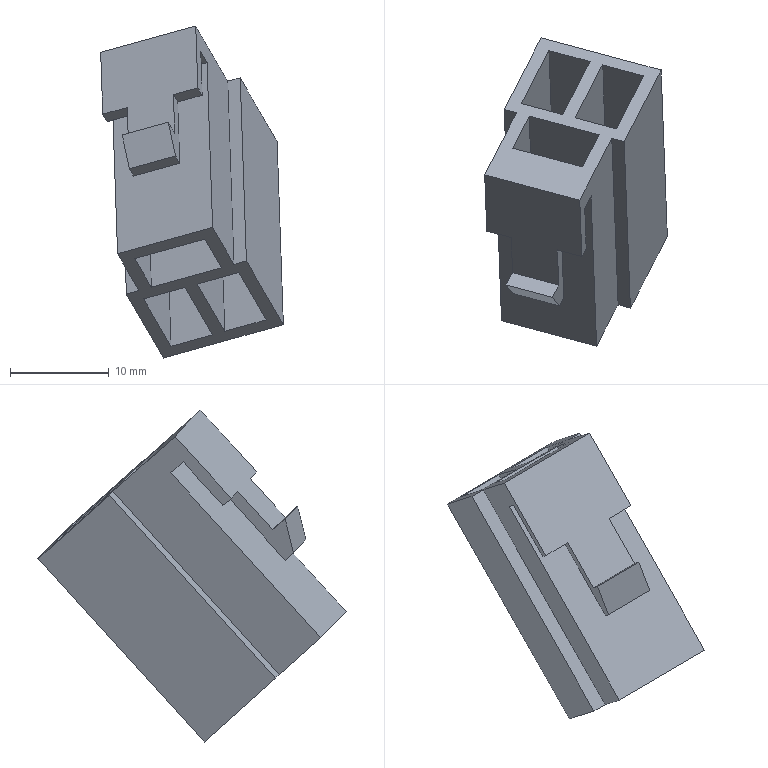Part | SolidWorks | features BaseBody 1 | 1 solid | 32 faces | box 18.462 x 31.146 x 33.559 mm | volume 2533 mm3 | plane 32
STEP:
#1=CARTESIAN_POINT('',(-173.307,-69.475,5.1));
#2=VERTEX_POINT('',#1);
#3=CARTESIAN_POINT('',(-173.175,-73.005,1.213));
#4=VERTEX_POINT('',#3);
#5=CARTESIAN_POINT('',(-173.175,-73.005,1.213));
#6=DIRECTION('',(0.02515,-0.6722,-0.7399));
#7=VECTOR('',#6,1000.);
#8=LINE('',#5,#7);
#9=EDGE_CURVE('',#2,#4,#8,.T.);
#10=ORIENTED_EDGE('',*,*,#9,.T.);
#11=CARTESIAN_POINT('',(-173.822,-74.26,2.331));
#12=VERTEX_POINT('',#11);
#13=CARTESIAN_POINT('',(-173.822,-74.26,2.331));
#14=DIRECTION('',(-0.359,-0.6969,0.6209));
#15=VECTOR('',#14,1000.);
#16=LINE('',#13,#15);
#17=EDGE_CURVE('',#4,#12,#16,.T.);
#18=ORIENTED_EDGE('',*,*,#17,.T.);
#19=CARTESIAN_POINT('',(-173.097,-75.101,-1.094));
#20=VERTEX_POINT('',#19);
#21=CARTESIAN_POINT('',(-173.097,-75.101,-1.094));
#22=DIRECTION('',(0.2013,-0.2337,-0.9513));
#23=VECTOR('',#22,1000.);
#24=LINE('',#21,#23);
#25=EDGE_CURVE('',#12,#20,#24,.T.);
#26=ORIENTED_EDGE('',*,*,#25,.T.);
#27=CARTESIAN_POINT('',(-172.666,-74.265,-1.839));
#28=VERTEX_POINT('',#27);
#29=CARTESIAN_POINT('',(-172.666,-74.265,-1.839));
#30=DIRECTION('',(0.359,0.6969,-0.6209));
#31=VECTOR('',#30,1000.);
#32=LINE('',#29,#31);
#33=EDGE_CURVE('',#20,#28,#32,.T.);
#34=ORIENTED_EDGE('',*,*,#33,.T.);
#35=CARTESIAN_POINT('',(-172.877,-68.639,4.355));
#36=VERTEX_POINT('',#35);
#37=CARTESIAN_POINT('',(-173.027,-64.617,8.781));
#38=DIRECTION('',(-0.02515,0.6722,0.7399));
#39=VECTOR('',#38,1000.);
#40=LINE('',#37,#39);
#41=EDGE_CURVE('',#28,#36,#40,.T.);
#42=ORIENTED_EDGE('',*,*,#41,.T.);
#43=CARTESIAN_POINT('',(-174.384,-71.565,6.963));
#44=DIRECTION('',(0.359,0.6969,-0.6209));
#45=VECTOR('',#44,1000.);
#46=LINE('',#43,#45);
#47=EDGE_CURVE('',#2,#36,#46,.T.);
#48=ORIENTED_EDGE('',*,*,#47,.F.);
#49=EDGE_LOOP('',(#10,#18,#26,#34,#42,#48));
#50=FACE_OUTER_BOUND('',#49,.T.);
#51=CARTESIAN_POINT('',(-174.103,-79.094,-1.325));
#52=DIRECTION('',(-0.933,0.25,-0.2588));
#53=DIRECTION('',(-0.2673,0.,0.9636));
#54=AXIS2_PLACEMENT_3D('',#51,#52,#53);
#55=PLANE('',#54);
#56=ADVANCED_FACE('',(#50),#55,.F.);
#57=CARTESIAN_POINT('',(-170.835,-70.137,5.786));
#58=VERTEX_POINT('',#57);
#59=CARTESIAN_POINT('',(-170.835,-70.137,5.786));
#60=DIRECTION('',(-0.933,0.25,-0.2588));
#61=VECTOR('',#60,1000.);
#62=LINE('',#59,#61);
#63=EDGE_CURVE('',#58,#2,#62,.T.);
#64=ORIENTED_EDGE('',*,*,#63,.T.);
#65=ORIENTED_EDGE('',*,*,#47,.T.);
#66=CARTESIAN_POINT('',(-170.404,-69.301,5.041));
#67=VERTEX_POINT('',#66);
#68=CARTESIAN_POINT('',(-170.404,-69.301,5.041));
#69=DIRECTION('',(0.933,-0.25,0.2588));
#70=VECTOR('',#69,1000.);
#71=LINE('',#68,#70);
#72=EDGE_CURVE('',#36,#67,#71,.T.);
#73=ORIENTED_EDGE('',*,*,#72,.T.);
#74=CARTESIAN_POINT('',(-169.758,-68.047,3.923));
#75=DIRECTION('',(0.359,0.6969,-0.6209));
#76=VECTOR('',#75,1000.);
#77=LINE('',#74,#76);
#78=EDGE_CURVE('',#58,#67,#77,.T.);
#79=ORIENTED_EDGE('',*,*,#78,.F.);
#80=EDGE_LOOP('',(#64,#65,#73,#79));
#81=FACE_OUTER_BOUND('',#80,.T.);
#82=CARTESIAN_POINT('',(-174.384,-71.565,6.963));
#83=DIRECTION('',(-0.02515,0.6722,0.7399));
#84=DIRECTION('',(0.9993,0.03738,0.));
#85=AXIS2_PLACEMENT_3D('',#82,#83,#84);
#86=PLANE('',#85);
#87=ADVANCED_FACE('',(#81),#86,.F.);
#88=CARTESIAN_POINT('',(-180.445,-67.562,3.12));
#89=VERTEX_POINT('',#88);
#90=CARTESIAN_POINT('',(-180.014,-66.726,2.375));
#91=VERTEX_POINT('',#90);
#92=CARTESIAN_POINT('',(-177.214,-61.29,-2.468));
#93=DIRECTION('',(0.359,0.6969,-0.6209));
#94=VECTOR('',#93,1000.);
#95=LINE('',#92,#94);
#96=EDGE_CURVE('',#89,#91,#95,.T.);
#97=ORIENTED_EDGE('',*,*,#96,.T.);
#98=CARTESIAN_POINT('',(-177.542,-67.389,3.061));
#99=VERTEX_POINT('',#98);
#100=CARTESIAN_POINT('',(-170.404,-69.301,5.041));
#101=DIRECTION('',(-0.933,0.25,-0.2588));
#102=VECTOR('',#101,1000.);
#103=LINE('',#100,#102);
#104=EDGE_CURVE('',#99,#91,#103,.T.);
#105=ORIENTED_EDGE('',*,*,#104,.F.);
#106=CARTESIAN_POINT('',(-177.973,-68.225,3.806));
#107=VERTEX_POINT('',#106);
#108=CARTESIAN_POINT('',(-179.049,-70.315,5.668));
#109=DIRECTION('',(0.359,0.6969,-0.6209));
#110=VECTOR('',#109,1000.);
#111=LINE('',#108,#110);
#112=EDGE_CURVE('',#107,#99,#111,.T.);
#113=ORIENTED_EDGE('',*,*,#112,.F.);
#114=CARTESIAN_POINT('',(-170.835,-70.137,5.786));
#115=DIRECTION('',(0.933,-0.25,0.2588));
#116=VECTOR('',#115,1000.);
#117=LINE('',#114,#116);
#118=EDGE_CURVE('',#89,#107,#117,.T.);
#119=ORIENTED_EDGE('',*,*,#118,.F.);
#120=EDGE_LOOP('',(#97,#105,#113,#119));
#121=FACE_OUTER_BOUND('',#120,.T.);
#122=CARTESIAN_POINT('',(-179.049,-70.315,5.668));
#123=DIRECTION('',(0.02515,-0.6722,-0.7399));
#124=DIRECTION('',(0.,-0.7402,0.6724));
#125=AXIS2_PLACEMENT_3D('',#122,#123,#124);
#126=PLANE('',#125);
#127=ADVANCED_FACE('',(#121),#126,.T.);
#128=ORIENTED_EDGE('',*,*,#112,.T.);
#129=CARTESIAN_POINT('',(-177.331,-73.015,-3.133));
#130=VERTEX_POINT('',#129);
#131=CARTESIAN_POINT('',(-177.692,-63.367,7.487));
#132=DIRECTION('',(-0.02515,0.6722,0.7399));
#133=VECTOR('',#132,1000.);
#134=LINE('',#131,#133);
#135=EDGE_CURVE('',#130,#99,#134,.T.);
#136=ORIENTED_EDGE('',*,*,#135,.F.);
#137=CARTESIAN_POINT('',(-177.762,-73.851,-2.388));
#138=VERTEX_POINT('',#137);
#139=CARTESIAN_POINT('',(-177.331,-73.015,-3.133));
#140=DIRECTION('',(0.359,0.6969,-0.6209));
#141=VECTOR('',#140,1000.);
#142=LINE('',#139,#141);
#143=EDGE_CURVE('',#138,#130,#142,.T.);
#144=ORIENTED_EDGE('',*,*,#143,.F.);
#145=CARTESIAN_POINT('',(-178.487,-73.01,1.037));
#146=VERTEX_POINT('',#145);
#147=CARTESIAN_POINT('',(-177.762,-73.851,-2.388));
#148=DIRECTION('',(0.2013,-0.2337,-0.9513));
#149=VECTOR('',#148,1000.);
#150=LINE('',#147,#149);
#151=EDGE_CURVE('',#146,#138,#150,.T.);
#152=ORIENTED_EDGE('',*,*,#151,.F.);
#153=CARTESIAN_POINT('',(-177.84,-71.755,-0.08074));
#154=VERTEX_POINT('',#153);
#155=CARTESIAN_POINT('',(-178.487,-73.01,1.037));
#156=DIRECTION('',(-0.359,-0.6969,0.6209));
#157=VECTOR('',#156,1000.);
#158=LINE('',#155,#157);
#159=EDGE_CURVE('',#154,#146,#158,.T.);
#160=ORIENTED_EDGE('',*,*,#159,.F.);
#161=CARTESIAN_POINT('',(-177.84,-71.755,-0.08074));
#162=DIRECTION('',(0.02515,-0.6722,-0.7399));
#163=VECTOR('',#162,1000.);
#164=LINE('',#161,#163);
#165=EDGE_CURVE('',#107,#154,#164,.T.);
#166=ORIENTED_EDGE('',*,*,#165,.F.);
#167=EDGE_LOOP('',(#128,#136,#144,#152,#160,#166));
#168=FACE_OUTER_BOUND('',#167,.T.);
#169=CARTESIAN_POINT('',(-178.768,-77.844,-2.619));
#170=DIRECTION('',(-0.933,0.25,-0.2588));
#171=DIRECTION('',(-0.2673,0.,0.9636));
#172=AXIS2_PLACEMENT_3D('',#169,#170,#171);
#173=PLANE('',#172);
#174=ADVANCED_FACE('',(#168),#173,.T.);
#175=CARTESIAN_POINT('',(-179.519,-61.45,5.684));
#176=VERTEX_POINT('',#175);
#177=CARTESIAN_POINT('',(-180.165,-62.705,6.801));
#178=VERTEX_POINT('',#177);
#179=CARTESIAN_POINT('',(-179.519,-61.45,5.684));
#180=DIRECTION('',(-0.359,-0.6969,0.6209));
#181=VECTOR('',#180,1000.);
#182=LINE('',#179,#181);
#183=EDGE_CURVE('',#176,#178,#182,.T.);
#184=ORIENTED_EDGE('',*,*,#183,.F.);
#185=CARTESIAN_POINT('',(-169.909,-64.025,8.35));
#186=VERTEX_POINT('',#185);
#187=CARTESIAN_POINT('',(-169.909,-64.025,8.35));
#188=DIRECTION('',(-0.933,0.25,-0.2588));
#189=VECTOR('',#188,1000.);
#190=LINE('',#187,#189);
#191=EDGE_CURVE('',#186,#176,#190,.T.);
#192=ORIENTED_EDGE('',*,*,#191,.F.);
#193=CARTESIAN_POINT('',(-170.555,-65.28,9.467));
#194=VERTEX_POINT('',#193);
#195=CARTESIAN_POINT('',(-169.909,-64.025,8.35));
#196=DIRECTION('',(-0.359,-0.6969,0.6209));
#197=VECTOR('',#196,1000.);
#198=LINE('',#195,#197);
#199=EDGE_CURVE('',#186,#194,#198,.T.);
#200=ORIENTED_EDGE('',*,*,#199,.T.);
#201=CARTESIAN_POINT('',(-170.555,-65.28,9.467));
#202=DIRECTION('',(-0.933,0.25,-0.2588));
#203=VECTOR('',#202,1000.);
#204=LINE('',#201,#203);
#205=EDGE_CURVE('',#194,#178,#204,.T.);
#206=ORIENTED_EDGE('',*,*,#205,.T.);
#207=EDGE_LOOP('',(#184,#192,#200,#206));
#208=FACE_OUTER_BOUND('',#207,.T.);
#209=CARTESIAN_POINT('',(-169.909,-64.025,8.35));
#210=DIRECTION('',(0.02515,-0.6722,-0.7399));
#211=DIRECTION('',(0.,-0.7402,0.6724));
#212=AXIS2_PLACEMENT_3D('',#209,#210,#211);
#213=PLANE('',#212);
#214=ADVANCED_FACE('',(#208),#213,.T.);
#215=CARTESIAN_POINT('',(-170.117,-77.892,-9.509));
#216=VERTEX_POINT('',#215);
#217=CARTESIAN_POINT('',(-168.448,-74.651,-12.396));
#218=VERTEX_POINT('',#217);
#219=CARTESIAN_POINT('',(-170.117,-77.892,-9.509));
#220=DIRECTION('',(0.359,0.6969,-0.6209));
#221=VECTOR('',#220,1000.);
#222=LINE('',#219,#221);
#223=EDGE_CURVE('',#216,#218,#222,.T.);
#224=ORIENTED_EDGE('',*,*,#223,.T.);
#225=CARTESIAN_POINT('',(-175.539,-72.751,-14.363));
#226=VERTEX_POINT('',#225);
#227=CARTESIAN_POINT('',(-168.448,-74.651,-12.396));
#228=DIRECTION('',(-0.933,0.25,-0.2588));
#229=VECTOR('',#228,1000.);
#230=LINE('',#227,#229);
#231=EDGE_CURVE('',#218,#226,#230,.T.);
#232=ORIENTED_EDGE('',*,*,#231,.T.);
#233=CARTESIAN_POINT('',(-177.208,-75.992,-11.476));
#234=VERTEX_POINT('',#233);
#235=CARTESIAN_POINT('',(-175.539,-72.751,-14.363));
#236=DIRECTION('',(-0.359,-0.6969,0.6209));
#237=VECTOR('',#236,1000.);
#238=LINE('',#235,#237);
#239=EDGE_CURVE('',#226,#234,#238,.T.);
#240=ORIENTED_EDGE('',*,*,#239,.T.);
#241=CARTESIAN_POINT('',(-177.208,-75.992,-11.476));
#242=DIRECTION('',(0.933,-0.25,0.2588));
#243=VECTOR('',#242,1000.);
#244=LINE('',#241,#243);
#245=EDGE_CURVE('',#234,#216,#244,.T.);
#246=ORIENTED_EDGE('',*,*,#245,.T.);
#247=EDGE_LOOP('',(#224,#232,#240,#246));
#248=FACE_BOUND('',#247,.T.);
#249=CARTESIAN_POINT('',(-169.374,-67.226,-19.173));
#250=VERTEX_POINT('',#249);
#251=CARTESIAN_POINT('',(-173.55,-66.107,-20.331));
#252=VERTEX_POINT('',#251);
#253=CARTESIAN_POINT('',(-169.374,-67.226,-19.173));
#254=DIRECTION('',(-0.933,0.25,-0.2588));
#255=VECTOR('',#254,1000.);
#256=LINE('',#253,#255);
#257=EDGE_CURVE('',#250,#252,#256,.T.);
#258=ORIENTED_EDGE('',*,*,#257,.T.);
#259=CARTESIAN_POINT('',(-176.314,-71.473,-15.551));
#260=VERTEX_POINT('',#259);
#261=CARTESIAN_POINT('',(-173.55,-66.107,-20.331));
#262=DIRECTION('',(-0.359,-0.6969,0.6209));
#263=VECTOR('',#262,1000.);
#264=LINE('',#261,#263);
#265=EDGE_CURVE('',#252,#260,#264,.T.);
#266=ORIENTED_EDGE('',*,*,#265,.T.);
#267=CARTESIAN_POINT('',(-172.138,-72.592,-14.392));
#268=VERTEX_POINT('',#267);
#269=CARTESIAN_POINT('',(-176.314,-71.473,-15.551));
#270=DIRECTION('',(0.933,-0.25,0.2588));
#271=VECTOR('',#270,1000.);
#272=LINE('',#269,#271);
#273=EDGE_CURVE('',#260,#268,#272,.T.);
#274=ORIENTED_EDGE('',*,*,#273,.T.);
#275=CARTESIAN_POINT('',(-172.138,-72.592,-14.392));
#276=DIRECTION('',(0.359,0.6969,-0.6209));
#277=VECTOR('',#276,1000.);
#278=LINE('',#275,#277);
#279=EDGE_CURVE('',#268,#250,#278,.T.);
#280=ORIENTED_EDGE('',*,*,#279,.T.);
#281=EDGE_LOOP('',(#258,#266,#274,#280));
#282=FACE_BOUND('',#281,.T.);
#283=CARTESIAN_POINT('',(-170.879,-72.929,-14.043));
#284=VERTEX_POINT('',#283);
#285=CARTESIAN_POINT('',(-166.704,-74.048,-12.885));
#286=VERTEX_POINT('',#285);
#287=CARTESIAN_POINT('',(-170.879,-72.929,-14.043));
#288=DIRECTION('',(0.933,-0.25,0.2588));
#289=VECTOR('',#288,1000.);
#290=LINE('',#287,#289);
#291=EDGE_CURVE('',#284,#286,#290,.T.);
#292=ORIENTED_EDGE('',*,*,#291,.T.);
#293=CARTESIAN_POINT('',(-163.94,-68.682,-17.665));
#294=VERTEX_POINT('',#293);
#295=CARTESIAN_POINT('',(-166.704,-74.048,-12.885));
#296=DIRECTION('',(0.359,0.6969,-0.6209));
#297=VECTOR('',#296,1000.);
#298=LINE('',#295,#297);
#299=EDGE_CURVE('',#286,#294,#298,.T.);
#300=ORIENTED_EDGE('',*,*,#299,.T.);
#301=CARTESIAN_POINT('',(-168.115,-67.563,-18.824));
#302=VERTEX_POINT('',#301);
#303=CARTESIAN_POINT('',(-163.94,-68.682,-17.665));
#304=DIRECTION('',(-0.933,0.25,-0.2588));
#305=VECTOR('',#304,1000.);
#306=LINE('',#303,#305);
#307=EDGE_CURVE('',#294,#302,#306,.T.);
#308=ORIENTED_EDGE('',*,*,#307,.T.);
#309=CARTESIAN_POINT('',(-168.115,-67.563,-18.824));
#310=DIRECTION('',(-0.359,-0.6969,0.6209));
#311=VECTOR('',#310,1000.);
#312=LINE('',#309,#311);
#313=EDGE_CURVE('',#302,#284,#312,.T.);
#314=ORIENTED_EDGE('',*,*,#313,.T.);
#315=EDGE_LOOP('',(#292,#300,#308,#314));
#316=FACE_BOUND('',#315,.T.);
#317=CARTESIAN_POINT('',(-167.188,-74.989,-12.046));
#318=VERTEX_POINT('',#317);
#319=CARTESIAN_POINT('',(-165.929,-75.326,-11.697));
#320=VERTEX_POINT('',#319);
#321=CARTESIAN_POINT('',(-167.188,-74.989,-12.046));
#322=DIRECTION('',(0.933,-0.25,0.2588));
#323=VECTOR('',#322,1000.);
#324=LINE('',#321,#323);
#325=EDGE_CURVE('',#318,#320,#324,.T.);
#326=ORIENTED_EDGE('',*,*,#325,.F.);
#327=CARTESIAN_POINT('',(-169.342,-79.17,-8.321));
#328=VERTEX_POINT('',#327);
#329=CARTESIAN_POINT('',(-169.342,-79.17,-8.321));
#330=DIRECTION('',(0.359,0.6969,-0.6209));
#331=VECTOR('',#330,1000.);
#332=LINE('',#329,#331);
#333=EDGE_CURVE('',#328,#318,#332,.T.);
#334=ORIENTED_EDGE('',*,*,#333,.F.);
#335=CARTESIAN_POINT('',(-178.952,-76.595,-10.987));
#336=VERTEX_POINT('',#335);
#337=CARTESIAN_POINT('',(-178.952,-76.595,-10.987));
#338=DIRECTION('',(0.933,-0.25,0.2588));
#339=VECTOR('',#338,1000.);
#340=LINE('',#337,#339);
#341=EDGE_CURVE('',#336,#328,#340,.T.);
#342=ORIENTED_EDGE('',*,*,#341,.F.);
#343=CARTESIAN_POINT('',(-176.798,-72.414,-14.712));
#344=VERTEX_POINT('',#343);
#345=CARTESIAN_POINT('',(-176.798,-72.414,-14.712));
#346=DIRECTION('',(-0.359,-0.6969,0.6209));
#347=VECTOR('',#346,1000.);
#348=LINE('',#345,#347);
#349=EDGE_CURVE('',#344,#336,#348,.T.);
#350=ORIENTED_EDGE('',*,*,#349,.F.);
#351=CARTESIAN_POINT('',(-178.058,-72.076,-15.062));
#352=VERTEX_POINT('',#351);
#353=CARTESIAN_POINT('',(-178.058,-72.076,-15.062));
#354=DIRECTION('',(0.933,-0.25,0.2588));
#355=VECTOR('',#354,1000.);
#356=LINE('',#353,#355);
#357=EDGE_CURVE('',#352,#344,#356,.T.);
#358=ORIENTED_EDGE('',*,*,#357,.F.);
#359=CARTESIAN_POINT('',(-174.325,-64.829,-21.519));
#360=VERTEX_POINT('',#359);
#361=CARTESIAN_POINT('',(-174.325,-64.829,-21.519));
#362=DIRECTION('',(-0.359,-0.6969,0.6209));
#363=VECTOR('',#362,1000.);
#364=LINE('',#361,#363);
#365=EDGE_CURVE('',#360,#352,#364,.T.);
#366=ORIENTED_EDGE('',*,*,#365,.F.);
#367=CARTESIAN_POINT('',(-162.195,-68.079,-18.154));
#368=VERTEX_POINT('',#367);
#369=CARTESIAN_POINT('',(-162.195,-68.079,-18.154));
#370=DIRECTION('',(-0.933,0.25,-0.2588));
#371=VECTOR('',#370,1000.);
#372=LINE('',#369,#371);
#373=EDGE_CURVE('',#368,#360,#372,.T.);
#374=ORIENTED_EDGE('',*,*,#373,.F.);
#375=CARTESIAN_POINT('',(-165.929,-75.326,-11.697));
#376=DIRECTION('',(0.359,0.6969,-0.6209));
#377=VECTOR('',#376,1000.);
#378=LINE('',#375,#377);
#379=EDGE_CURVE('',#320,#368,#378,.T.);
#380=ORIENTED_EDGE('',*,*,#379,.F.);
#381=EDGE_LOOP('',(#326,#334,#342,#350,#358,#366,#374,#380));
#382=FACE_OUTER_BOUND('',#381,.T.);
#383=CARTESIAN_POINT('',(-178.736,-73.084,-14.169));
#384=DIRECTION('',(0.02515,-0.6722,-0.7399));
#385=DIRECTION('',(0.,-0.7402,0.6724));
#386=AXIS2_PLACEMENT_3D('',#383,#384,#385);
#387=PLANE('',#386);
#388=ADVANCED_FACE('',(#248,#282,#316,#382),#387,.T.);
#389=CARTESIAN_POINT('',(-170.746,-61.087,8.99));
#390=VERTEX_POINT('',#389);
#391=CARTESIAN_POINT('',(-169.076,-57.846,6.103));
#392=VERTEX_POINT('',#391);
#393=CARTESIAN_POINT('',(-170.746,-61.087,8.99));
#394=DIRECTION('',(0.359,0.6969,-0.6209));
#395=VECTOR('',#394,1000.);
#396=LINE('',#393,#395);
#397=EDGE_CURVE('',#390,#392,#396,.T.);
#398=ORIENTED_EDGE('',*,*,#397,.F.);
#399=CARTESIAN_POINT('',(-177.837,-59.187,7.023));
#400=VERTEX_POINT('',#399);
#401=CARTESIAN_POINT('',(-177.837,-59.187,7.023));
#402=DIRECTION('',(0.933,-0.25,0.2588));
#403=VECTOR('',#402,1000.);
#404=LINE('',#401,#403);
#405=EDGE_CURVE('',#400,#390,#404,.T.);
#406=ORIENTED_EDGE('',*,*,#405,.F.);
#407=CARTESIAN_POINT('',(-176.167,-55.946,4.136));
#408=VERTEX_POINT('',#407);
#409=CARTESIAN_POINT('',(-176.167,-55.946,4.136));
#410=DIRECTION('',(-0.359,-0.6969,0.6209));
#411=VECTOR('',#410,1000.);
#412=LINE('',#409,#411);
#413=EDGE_CURVE('',#408,#400,#412,.T.);
#414=ORIENTED_EDGE('',*,*,#413,.F.);
#415=CARTESIAN_POINT('',(-169.076,-57.846,6.103));
#416=DIRECTION('',(-0.933,0.25,-0.2588));
#417=VECTOR('',#416,1000.);
#418=LINE('',#415,#417);
#419=EDGE_CURVE('',#392,#408,#418,.T.);
#420=ORIENTED_EDGE('',*,*,#419,.F.);
#421=EDGE_LOOP('',(#398,#406,#414,#420));
#422=FACE_BOUND('',#421,.T.);
#423=CARTESIAN_POINT('',(-170.003,-50.421,-0.6745));
#424=VERTEX_POINT('',#423);
#425=CARTESIAN_POINT('',(-174.178,-49.302,-1.833));
#426=VERTEX_POINT('',#425);
#427=CARTESIAN_POINT('',(-170.003,-50.421,-0.6745));
#428=DIRECTION('',(-0.933,0.25,-0.2588));
#429=VECTOR('',#428,1000.);
#430=LINE('',#427,#429);
#431=EDGE_CURVE('',#424,#426,#430,.T.);
#432=ORIENTED_EDGE('',*,*,#431,.F.);
#433=CARTESIAN_POINT('',(-172.767,-55.787,4.106));
#434=VERTEX_POINT('',#433);
#435=CARTESIAN_POINT('',(-172.767,-55.787,4.106));
#436=DIRECTION('',(0.359,0.6969,-0.6209));
#437=VECTOR('',#436,1000.);
#438=LINE('',#435,#437);
#439=EDGE_CURVE('',#434,#424,#438,.T.);
#440=ORIENTED_EDGE('',*,*,#439,.F.);
#441=CARTESIAN_POINT('',(-176.942,-54.668,2.948));
#442=VERTEX_POINT('',#441);
#443=CARTESIAN_POINT('',(-176.942,-54.668,2.948));
#444=DIRECTION('',(0.933,-0.25,0.2588));
#445=VECTOR('',#444,1000.);
#446=LINE('',#443,#445);
#447=EDGE_CURVE('',#442,#434,#446,.T.);
#448=ORIENTED_EDGE('',*,*,#447,.F.);
#449=CARTESIAN_POINT('',(-174.178,-49.302,-1.833));
#450=DIRECTION('',(-0.359,-0.6969,0.6209));
#451=VECTOR('',#450,1000.);
#452=LINE('',#449,#451);
#453=EDGE_CURVE('',#426,#442,#452,.T.);
#454=ORIENTED_EDGE('',*,*,#453,.F.);
#455=EDGE_LOOP('',(#432,#440,#448,#454));
#456=FACE_BOUND('',#455,.T.);
#457=CARTESIAN_POINT('',(-171.507,-56.124,4.456));
#458=VERTEX_POINT('',#457);
#459=CARTESIAN_POINT('',(-167.332,-57.243,5.614));
#460=VERTEX_POINT('',#459);
#461=CARTESIAN_POINT('',(-171.507,-56.124,4.456));
#462=DIRECTION('',(0.933,-0.25,0.2588));
#463=VECTOR('',#462,1000.);
#464=LINE('',#461,#463);
#465=EDGE_CURVE('',#458,#460,#464,.T.);
#466=ORIENTED_EDGE('',*,*,#465,.F.);
#467=CARTESIAN_POINT('',(-168.743,-50.758,-0.3251));
#468=VERTEX_POINT('',#467);
#469=CARTESIAN_POINT('',(-168.743,-50.758,-0.3251));
#470=DIRECTION('',(-0.359,-0.6969,0.6209));
#471=VECTOR('',#470,1000.);
#472=LINE('',#469,#471);
#473=EDGE_CURVE('',#468,#458,#472,.T.);
#474=ORIENTED_EDGE('',*,*,#473,.F.);
#475=CARTESIAN_POINT('',(-164.568,-51.877,0.8331));
#476=VERTEX_POINT('',#475);
#477=CARTESIAN_POINT('',(-164.568,-51.877,0.8331));
#478=DIRECTION('',(-0.933,0.25,-0.2588));
#479=VECTOR('',#478,1000.);
#480=LINE('',#477,#479);
#481=EDGE_CURVE('',#476,#468,#480,.T.);
#482=ORIENTED_EDGE('',*,*,#481,.F.);
#483=CARTESIAN_POINT('',(-167.332,-57.243,5.614));
#484=DIRECTION('',(0.359,0.6969,-0.6209));
#485=VECTOR('',#484,1000.);
#486=LINE('',#483,#485);
#487=EDGE_CURVE('',#460,#476,#486,.T.);
#488=ORIENTED_EDGE('',*,*,#487,.F.);
#489=EDGE_LOOP('',(#466,#474,#482,#488));
#490=FACE_BOUND('',#489,.T.);
#491=CARTESIAN_POINT('',(-167.817,-58.184,6.452));
#492=VERTEX_POINT('',#491);
#493=CARTESIAN_POINT('',(-166.557,-58.521,6.801));
#494=VERTEX_POINT('',#493);
#495=CARTESIAN_POINT('',(-167.817,-58.184,6.452));
#496=DIRECTION('',(0.933,-0.25,0.2588));
#497=VECTOR('',#496,1000.);
#498=LINE('',#495,#497);
#499=EDGE_CURVE('',#492,#494,#498,.T.);
#500=ORIENTED_EDGE('',*,*,#499,.T.);
#501=CARTESIAN_POINT('',(-162.824,-51.273,0.3443));
#502=VERTEX_POINT('',#501);
#503=CARTESIAN_POINT('',(-166.557,-58.521,6.801));
#504=DIRECTION('',(0.359,0.6969,-0.6209));
#505=VECTOR('',#504,1000.);
#506=LINE('',#503,#505);
#507=EDGE_CURVE('',#494,#502,#506,.T.);
#508=ORIENTED_EDGE('',*,*,#507,.T.);
#509=CARTESIAN_POINT('',(-174.953,-48.023,-3.02));
#510=VERTEX_POINT('',#509);
#511=CARTESIAN_POINT('',(-162.824,-51.273,0.3443));
#512=DIRECTION('',(-0.933,0.25,-0.2588));
#513=VECTOR('',#512,1000.);
#514=LINE('',#511,#513);
#515=EDGE_CURVE('',#502,#510,#514,.T.);
#516=ORIENTED_EDGE('',*,*,#515,.T.);
#517=CARTESIAN_POINT('',(-178.686,-55.271,3.437));
#518=VERTEX_POINT('',#517);
#519=CARTESIAN_POINT('',(-174.953,-48.023,-3.02));
#520=DIRECTION('',(-0.359,-0.6969,0.6209));
#521=VECTOR('',#520,1000.);
#522=LINE('',#519,#521);
#523=EDGE_CURVE('',#510,#518,#522,.T.);
#524=ORIENTED_EDGE('',*,*,#523,.T.);
#525=CARTESIAN_POINT('',(-177.427,-55.609,3.786));
#526=VERTEX_POINT('',#525);
#527=CARTESIAN_POINT('',(-178.686,-55.271,3.437));
#528=DIRECTION('',(0.933,-0.25,0.2588));
#529=VECTOR('',#528,1000.);
#530=LINE('',#527,#529);
#531=EDGE_CURVE('',#518,#526,#530,.T.);
#532=ORIENTED_EDGE('',*,*,#531,.T.);
#533=CARTESIAN_POINT('',(-180.658,-61.881,9.374));
#534=VERTEX_POINT('',#533);
#535=CARTESIAN_POINT('',(-177.427,-55.609,3.786));
#536=DIRECTION('',(-0.359,-0.6969,0.6209));
#537=VECTOR('',#536,1000.);
#538=LINE('',#535,#537);
#539=EDGE_CURVE('',#526,#534,#538,.T.);
#540=ORIENTED_EDGE('',*,*,#539,.T.);
#541=CARTESIAN_POINT('',(-171.048,-64.456,12.04));
#542=VERTEX_POINT('',#541);
#543=CARTESIAN_POINT('',(-171.048,-64.456,12.04));
#544=DIRECTION('',(-0.933,0.25,-0.2588));
#545=VECTOR('',#544,1000.);
#546=LINE('',#543,#545);
#547=EDGE_CURVE('',#542,#534,#546,.T.);
#548=ORIENTED_EDGE('',*,*,#547,.F.);
#549=CARTESIAN_POINT('',(-169.971,-62.365,10.177));
#550=DIRECTION('',(0.359,0.6969,-0.6209));
#551=VECTOR('',#550,1000.);
#552=LINE('',#549,#551);
#553=EDGE_CURVE('',#542,#492,#552,.T.);
#554=ORIENTED_EDGE('',*,*,#553,.T.);
#555=EDGE_LOOP('',(#500,#508,#516,#524,#532,#540,#548,#554));
#556=FACE_OUTER_BOUND('',#555,.T.);
#557=CARTESIAN_POINT('',(-179.365,-56.279,4.329));
#558=DIRECTION('',(0.02515,-0.6722,-0.7399));
#559=DIRECTION('',(0.,-0.7402,0.6724));
#560=AXIS2_PLACEMENT_3D('',#557,#558,#559);
#561=PLANE('',#560);
#562=ADVANCED_FACE('',(#422,#456,#490,#556),#561,.F.);
#563=ORIENTED_EDGE('',*,*,#231,.F.);
#564=CARTESIAN_POINT('',(-169.897,-35.899,30.262));
#565=DIRECTION('',(0.02515,-0.6722,-0.7399));
#566=VECTOR('',#565,1000.);
#567=LINE('',#564,#566);
#568=EDGE_CURVE('',#392,#218,#567,.T.);
#569=ORIENTED_EDGE('',*,*,#568,.F.);
#570=ORIENTED_EDGE('',*,*,#419,.T.);
#571=CARTESIAN_POINT('',(-176.988,-33.999,28.295));
#572=DIRECTION('',(0.02515,-0.6722,-0.7399));
#573=VECTOR('',#572,1000.);
#574=LINE('',#571,#573);
#575=EDGE_CURVE('',#408,#226,#574,.T.);
#576=ORIENTED_EDGE('',*,*,#575,.T.);
#577=EDGE_LOOP('',(#563,#569,#570,#576));
#578=FACE_OUTER_BOUND('',#577,.T.);
#579=CARTESIAN_POINT('',(-169.897,-35.899,30.262));
#580=DIRECTION('',(-0.359,-0.6969,0.6209));
#581=DIRECTION('',(-0.889,0.4579,0.));
#582=AXIS2_PLACEMENT_3D('',#579,#580,#581);
#583=PLANE('',#582);
#584=ADVANCED_FACE('',(#578),#583,.T.);
#585=CARTESIAN_POINT('',(-170.703,-73.668,1.899));
#586=DIRECTION('',(-0.02515,0.6722,0.7399));
#587=VECTOR('',#586,1000.);
#588=LINE('',#585,#587);
#589=EDGE_CURVE('',#58,#542,#588,.T.);
#590=ORIENTED_EDGE('',*,*,#589,.F.);
#591=ORIENTED_EDGE('',*,*,#78,.T.);
#592=CARTESIAN_POINT('',(-170.555,-65.28,9.467));
#593=DIRECTION('',(0.02515,-0.6722,-0.7399));
#594=VECTOR('',#593,1000.);
#595=LINE('',#592,#594);
#596=EDGE_CURVE('',#194,#67,#595,.T.);
#597=ORIENTED_EDGE('',*,*,#596,.F.);
#598=ORIENTED_EDGE('',*,*,#199,.F.);
#599=CARTESIAN_POINT('',(-170.792,-40.418,34.337));
#600=DIRECTION('',(0.02515,-0.6722,-0.7399));
#601=VECTOR('',#600,1000.);
#602=LINE('',#599,#601);
#603=EDGE_CURVE('',#186,#328,#602,.T.);
#604=ORIENTED_EDGE('',*,*,#603,.T.);
#605=ORIENTED_EDGE('',*,*,#333,.T.);
#606=CARTESIAN_POINT('',(-168.638,-36.236,30.611));
#607=DIRECTION('',(0.02515,-0.6722,-0.7399));
#608=VECTOR('',#607,1000.);
#609=LINE('',#606,#608);
#610=EDGE_CURVE('',#492,#318,#609,.T.);
#611=ORIENTED_EDGE('',*,*,#610,.F.);
#612=ORIENTED_EDGE('',*,*,#553,.F.);
#613=EDGE_LOOP('',(#590,#591,#597,#598,#604,#605,#611,#612));
#614=FACE_OUTER_BOUND('',#613,.T.);
#615=CARTESIAN_POINT('',(-170.792,-40.418,34.337));
#616=DIRECTION('',(-0.933,0.25,-0.2588));
#617=DIRECTION('',(-0.2673,0.,0.9636));
#618=AXIS2_PLACEMENT_3D('',#615,#616,#617);
#619=PLANE('',#618);
#620=ADVANCED_FACE('',(#614),#619,.F.);
#621=ORIENTED_EDGE('',*,*,#299,.F.);
#622=CARTESIAN_POINT('',(-168.153,-35.295,29.773));
#623=DIRECTION('',(0.02515,-0.6722,-0.7399));
#624=VECTOR('',#623,1000.);
#625=LINE('',#622,#624);
#626=EDGE_CURVE('',#460,#286,#625,.T.);
#627=ORIENTED_EDGE('',*,*,#626,.F.);
#628=ORIENTED_EDGE('',*,*,#487,.T.);
#629=CARTESIAN_POINT('',(-165.389,-29.929,24.992));
#630=DIRECTION('',(0.02515,-0.6722,-0.7399));
#631=VECTOR('',#630,1000.);
#632=LINE('',#629,#631);
#633=EDGE_CURVE('',#476,#294,#632,.T.);
#634=ORIENTED_EDGE('',*,*,#633,.T.);
#635=EDGE_LOOP('',(#621,#627,#628,#634));
#636=FACE_OUTER_BOUND('',#635,.T.);
#637=CARTESIAN_POINT('',(-168.153,-35.295,29.773));
#638=DIRECTION('',(-0.933,0.25,-0.2588));
#639=DIRECTION('',(-0.2673,0.,0.9636));
#640=AXIS2_PLACEMENT_3D('',#637,#638,#639);
#641=PLANE('',#640);
#642=ADVANCED_FACE('',(#636),#641,.T.);
#643=ORIENTED_EDGE('',*,*,#265,.F.);
#644=CARTESIAN_POINT('',(-174.999,-27.354,22.326));
#645=DIRECTION('',(0.02515,-0.6722,-0.7399));
#646=VECTOR('',#645,1000.);
#647=LINE('',#644,#646);
#648=EDGE_CURVE('',#426,#252,#647,.T.);
#649=ORIENTED_EDGE('',*,*,#648,.F.);
#650=ORIENTED_EDGE('',*,*,#453,.T.);
#651=CARTESIAN_POINT('',(-177.763,-32.72,27.107));
#652=DIRECTION('',(0.02515,-0.6722,-0.7399));
#653=VECTOR('',#652,1000.);
#654=LINE('',#651,#653);
#655=EDGE_CURVE('',#442,#260,#654,.T.);
#656=ORIENTED_EDGE('',*,*,#655,.T.);
#657=EDGE_LOOP('',(#643,#649,#650,#656));
#658=FACE_OUTER_BOUND('',#657,.T.);
#659=CARTESIAN_POINT('',(-174.999,-27.354,22.326));
#660=DIRECTION('',(0.933,-0.25,0.2588));
#661=DIRECTION('',(0.,-0.7193,-0.6947));
#662=AXIS2_PLACEMENT_3D('',#659,#660,#661);
#663=PLANE('',#662);
#664=ADVANCED_FACE('',(#658),#663,.T.);
#665=ORIENTED_EDGE('',*,*,#341,.T.);
#666=ORIENTED_EDGE('',*,*,#603,.F.);
#667=ORIENTED_EDGE('',*,*,#191,.T.);
#668=CARTESIAN_POINT('',(-180.402,-37.843,31.671));
#669=DIRECTION('',(0.02515,-0.6722,-0.7399));
#670=VECTOR('',#669,1000.);
#671=LINE('',#668,#670);
#672=EDGE_CURVE('',#176,#336,#671,.T.);
#673=ORIENTED_EDGE('',*,*,#672,.T.);
#674=EDGE_LOOP('',(#665,#666,#667,#673));
#675=FACE_OUTER_BOUND('',#674,.T.);
#676=CARTESIAN_POINT('',(-180.402,-37.843,31.671));
#677=DIRECTION('',(0.359,0.6969,-0.6209));
#678=DIRECTION('',(-0.8657,0.,-0.5005));
#679=AXIS2_PLACEMENT_3D('',#676,#677,#678);
#680=PLANE('',#679);
#681=ADVANCED_FACE('',(#675),#680,.F.);
#682=ORIENTED_EDGE('',*,*,#357,.T.);
#683=CARTESIAN_POINT('',(-178.248,-33.661,27.945));
#684=DIRECTION('',(0.02515,-0.6722,-0.7399));
#685=VECTOR('',#684,1000.);
#686=LINE('',#683,#685);
#687=EDGE_CURVE('',#526,#344,#686,.T.);
#688=ORIENTED_EDGE('',*,*,#687,.F.);
#689=ORIENTED_EDGE('',*,*,#531,.F.);
#690=CARTESIAN_POINT('',(-179.507,-33.324,27.596));
#691=DIRECTION('',(0.02515,-0.6722,-0.7399));
#692=VECTOR('',#691,1000.);
#693=LINE('',#690,#692);
#694=EDGE_CURVE('',#518,#352,#693,.T.);
#695=ORIENTED_EDGE('',*,*,#694,.T.);
#696=EDGE_LOOP('',(#682,#688,#689,#695));
#697=FACE_OUTER_BOUND('',#696,.T.);
#698=CARTESIAN_POINT('',(-179.507,-33.324,27.596));
#699=DIRECTION('',(0.359,0.6969,-0.6209));
#700=DIRECTION('',(-0.8657,0.,-0.5005));
#701=AXIS2_PLACEMENT_3D('',#698,#699,#700);
#702=PLANE('',#701);
#703=ADVANCED_FACE('',(#697),#702,.F.);
#704=ORIENTED_EDGE('',*,*,#365,.T.);
#705=ORIENTED_EDGE('',*,*,#694,.F.);
#706=ORIENTED_EDGE('',*,*,#523,.F.);
#707=CARTESIAN_POINT('',(-175.774,-26.076,21.139));
#708=DIRECTION('',(0.02515,-0.6722,-0.7399));
#709=VECTOR('',#708,1000.);
#710=LINE('',#707,#709);
#711=EDGE_CURVE('',#510,#360,#710,.T.);
#712=ORIENTED_EDGE('',*,*,#711,.T.);
#713=EDGE_LOOP('',(#704,#705,#706,#712));
#714=FACE_OUTER_BOUND('',#713,.T.);
#715=CARTESIAN_POINT('',(-175.774,-26.076,21.139));
#716=DIRECTION('',(0.933,-0.25,0.2588));
#717=DIRECTION('',(0.,-0.7193,-0.6947));
#718=AXIS2_PLACEMENT_3D('',#715,#716,#717);
#719=PLANE('',#718);
#720=ADVANCED_FACE('',(#714),#719,.F.);
#721=ORIENTED_EDGE('',*,*,#373,.T.);
#722=ORIENTED_EDGE('',*,*,#711,.F.);
#723=ORIENTED_EDGE('',*,*,#515,.F.);
#724=CARTESIAN_POINT('',(-163.645,-29.326,24.503));
#725=DIRECTION('',(0.02515,-0.6722,-0.7399));
#726=VECTOR('',#725,1000.);
#727=LINE('',#724,#726);
#728=EDGE_CURVE('',#502,#368,#727,.T.);
#729=ORIENTED_EDGE('',*,*,#728,.T.);
#730=EDGE_LOOP('',(#721,#722,#723,#729));
#731=FACE_OUTER_BOUND('',#730,.T.);
#732=CARTESIAN_POINT('',(-163.645,-29.326,24.503));
#733=DIRECTION('',(-0.359,-0.6969,0.6209));
#734=DIRECTION('',(-0.889,0.4579,0.));
#735=AXIS2_PLACEMENT_3D('',#732,#733,#734);
#736=PLANE('',#735);
#737=ADVANCED_FACE('',(#731),#736,.F.);
#738=ORIENTED_EDGE('',*,*,#379,.T.);
#739=ORIENTED_EDGE('',*,*,#728,.F.);
#740=ORIENTED_EDGE('',*,*,#507,.F.);
#741=CARTESIAN_POINT('',(-167.378,-36.574,30.961));
#742=DIRECTION('',(0.02515,-0.6722,-0.7399));
#743=VECTOR('',#742,1000.);
#744=LINE('',#741,#743);
#745=EDGE_CURVE('',#494,#320,#744,.T.);
#746=ORIENTED_EDGE('',*,*,#745,.T.);
#747=EDGE_LOOP('',(#738,#739,#740,#746));
#748=FACE_OUTER_BOUND('',#747,.T.);
#749=CARTESIAN_POINT('',(-167.378,-36.574,30.961));
#750=DIRECTION('',(-0.933,0.25,-0.2588));
#751=DIRECTION('',(-0.2673,0.,0.9636));
#752=AXIS2_PLACEMENT_3D('',#749,#750,#751);
#753=PLANE('',#752);
#754=ADVANCED_FACE('',(#748),#753,.F.);
#755=ORIENTED_EDGE('',*,*,#325,.T.);
#756=ORIENTED_EDGE('',*,*,#745,.F.);
#757=ORIENTED_EDGE('',*,*,#499,.F.);
#758=ORIENTED_EDGE('',*,*,#610,.T.);
#759=EDGE_LOOP('',(#755,#756,#757,#758));
#760=FACE_OUTER_BOUND('',#759,.T.);
#761=CARTESIAN_POINT('',(-168.638,-36.236,30.611));
#762=DIRECTION('',(0.359,0.6969,-0.6209));
#763=DIRECTION('',(-0.8657,0.,-0.5005));
#764=AXIS2_PLACEMENT_3D('',#761,#762,#763);
#765=PLANE('',#764);
#766=ADVANCED_FACE('',(#760),#765,.F.);
#767=ORIENTED_EDGE('',*,*,#307,.F.);
#768=ORIENTED_EDGE('',*,*,#633,.F.);
#769=ORIENTED_EDGE('',*,*,#481,.T.);
#770=CARTESIAN_POINT('',(-169.564,-28.811,23.834));
#771=DIRECTION('',(0.02515,-0.6722,-0.7399));
#772=VECTOR('',#771,1000.);
#773=LINE('',#770,#772);
#774=EDGE_CURVE('',#468,#302,#773,.T.);
#775=ORIENTED_EDGE('',*,*,#774,.T.);
#776=EDGE_LOOP('',(#767,#768,#769,#775));
#777=FACE_OUTER_BOUND('',#776,.T.);
#778=CARTESIAN_POINT('',(-165.389,-29.929,24.992));
#779=DIRECTION('',(-0.359,-0.6969,0.6209));
#780=DIRECTION('',(-0.889,0.4579,0.));
#781=AXIS2_PLACEMENT_3D('',#778,#779,#780);
#782=PLANE('',#781);
#783=ADVANCED_FACE('',(#777),#782,.T.);
#784=ORIENTED_EDGE('',*,*,#313,.F.);
#785=ORIENTED_EDGE('',*,*,#774,.F.);
#786=ORIENTED_EDGE('',*,*,#473,.T.);
#787=CARTESIAN_POINT('',(-172.328,-34.177,28.615));
#788=DIRECTION('',(0.02515,-0.6722,-0.7399));
#789=VECTOR('',#788,1000.);
#790=LINE('',#787,#789);
#791=EDGE_CURVE('',#458,#284,#790,.T.);
#792=ORIENTED_EDGE('',*,*,#791,.T.);
#793=EDGE_LOOP('',(#784,#785,#786,#792));
#794=FACE_OUTER_BOUND('',#793,.T.);
#795=CARTESIAN_POINT('',(-169.564,-28.811,23.834));
#796=DIRECTION('',(0.933,-0.25,0.2588));
#797=DIRECTION('',(0.,-0.7193,-0.6947));
#798=AXIS2_PLACEMENT_3D('',#795,#796,#797);
#799=PLANE('',#798);
#800=ADVANCED_FACE('',(#794),#799,.T.);
#801=ORIENTED_EDGE('',*,*,#291,.F.);
#802=ORIENTED_EDGE('',*,*,#791,.F.);
#803=ORIENTED_EDGE('',*,*,#465,.T.);
#804=ORIENTED_EDGE('',*,*,#626,.T.);
#805=EDGE_LOOP('',(#801,#802,#803,#804));
#806=FACE_OUTER_BOUND('',#805,.T.);
#807=CARTESIAN_POINT('',(-172.328,-34.177,28.615));
#808=DIRECTION('',(0.359,0.6969,-0.6209));
#809=DIRECTION('',(-0.8657,0.,-0.5005));
#810=AXIS2_PLACEMENT_3D('',#807,#808,#809);
#811=PLANE('',#810);
#812=ADVANCED_FACE('',(#806),#811,.T.);
#813=ORIENTED_EDGE('',*,*,#273,.F.);
#814=ORIENTED_EDGE('',*,*,#655,.F.);
#815=ORIENTED_EDGE('',*,*,#447,.T.);
#816=CARTESIAN_POINT('',(-173.588,-33.839,28.265));
#817=DIRECTION('',(0.02515,-0.6722,-0.7399));
#818=VECTOR('',#817,1000.);
#819=LINE('',#816,#818);
#820=EDGE_CURVE('',#434,#268,#819,.T.);
#821=ORIENTED_EDGE('',*,*,#820,.T.);
#822=EDGE_LOOP('',(#813,#814,#815,#821));
#823=FACE_OUTER_BOUND('',#822,.T.);
#824=CARTESIAN_POINT('',(-177.763,-32.72,27.107));
#825=DIRECTION('',(0.359,0.6969,-0.6209));
#826=DIRECTION('',(-0.8657,0.,-0.5005));
#827=AXIS2_PLACEMENT_3D('',#824,#825,#826);
#828=PLANE('',#827);
#829=ADVANCED_FACE('',(#823),#828,.T.);
#830=ORIENTED_EDGE('',*,*,#279,.F.);
#831=ORIENTED_EDGE('',*,*,#820,.F.);
#832=ORIENTED_EDGE('',*,*,#439,.T.);
#833=CARTESIAN_POINT('',(-170.824,-28.473,23.485));
#834=DIRECTION('',(0.02515,-0.6722,-0.7399));
#835=VECTOR('',#834,1000.);
#836=LINE('',#833,#835);
#837=EDGE_CURVE('',#424,#250,#836,.T.);
#838=ORIENTED_EDGE('',*,*,#837,.T.);
#839=EDGE_LOOP('',(#830,#831,#832,#838));
#840=FACE_OUTER_BOUND('',#839,.T.);
#841=CARTESIAN_POINT('',(-173.588,-33.839,28.265));
#842=DIRECTION('',(-0.933,0.25,-0.2588));
#843=DIRECTION('',(-0.2673,0.,0.9636));
#844=AXIS2_PLACEMENT_3D('',#841,#842,#843);
#845=PLANE('',#844);
#846=ADVANCED_FACE('',(#840),#845,.T.);
#847=ORIENTED_EDGE('',*,*,#257,.F.);
#848=ORIENTED_EDGE('',*,*,#837,.F.);
#849=ORIENTED_EDGE('',*,*,#431,.T.);
#850=ORIENTED_EDGE('',*,*,#648,.T.);
#851=EDGE_LOOP('',(#847,#848,#849,#850));
#852=FACE_OUTER_BOUND('',#851,.T.);
#853=CARTESIAN_POINT('',(-170.824,-28.473,23.485));
#854=DIRECTION('',(-0.359,-0.6969,0.6209));
#855=DIRECTION('',(-0.889,0.4579,0.));
#856=AXIS2_PLACEMENT_3D('',#853,#854,#855);
#857=PLANE('',#856);
#858=ADVANCED_FACE('',(#852),#857,.T.);
#859=ORIENTED_EDGE('',*,*,#239,.F.);
#860=ORIENTED_EDGE('',*,*,#575,.F.);
#861=ORIENTED_EDGE('',*,*,#413,.T.);
#862=CARTESIAN_POINT('',(-178.658,-37.239,31.182));
#863=DIRECTION('',(0.02515,-0.6722,-0.7399));
#864=VECTOR('',#863,1000.);
#865=LINE('',#862,#864);
#866=EDGE_CURVE('',#400,#234,#865,.T.);
#867=ORIENTED_EDGE('',*,*,#866,.T.);
#868=EDGE_LOOP('',(#859,#860,#861,#867));
#869=FACE_OUTER_BOUND('',#868,.T.);
#870=CARTESIAN_POINT('',(-176.988,-33.999,28.295));
#871=DIRECTION('',(0.933,-0.25,0.2588));
#872=DIRECTION('',(0.,-0.7193,-0.6947));
#873=AXIS2_PLACEMENT_3D('',#870,#871,#872);
#874=PLANE('',#873);
#875=ADVANCED_FACE('',(#869),#874,.T.);
#876=ORIENTED_EDGE('',*,*,#245,.F.);
#877=ORIENTED_EDGE('',*,*,#866,.F.);
#878=ORIENTED_EDGE('',*,*,#405,.T.);
#879=CARTESIAN_POINT('',(-171.567,-39.139,33.149));
#880=DIRECTION('',(0.02515,-0.6722,-0.7399));
#881=VECTOR('',#880,1000.);
#882=LINE('',#879,#881);
#883=EDGE_CURVE('',#390,#216,#882,.T.);
#884=ORIENTED_EDGE('',*,*,#883,.T.);
#885=EDGE_LOOP('',(#876,#877,#878,#884));
#886=FACE_OUTER_BOUND('',#885,.T.);
#887=CARTESIAN_POINT('',(-178.658,-37.239,31.182));
#888=DIRECTION('',(0.359,0.6969,-0.6209));
#889=DIRECTION('',(-0.8657,0.,-0.5005));
#890=AXIS2_PLACEMENT_3D('',#887,#888,#889);
#891=PLANE('',#890);
#892=ADVANCED_FACE('',(#886),#891,.T.);
#893=ORIENTED_EDGE('',*,*,#223,.F.);
#894=ORIENTED_EDGE('',*,*,#883,.F.);
#895=ORIENTED_EDGE('',*,*,#397,.T.);
#896=ORIENTED_EDGE('',*,*,#568,.T.);
#897=EDGE_LOOP('',(#893,#894,#895,#896));
#898=FACE_OUTER_BOUND('',#897,.T.);
#899=CARTESIAN_POINT('',(-171.567,-39.139,33.149));
#900=DIRECTION('',(-0.933,0.25,-0.2588));
#901=DIRECTION('',(-0.2673,0.,0.9636));
#902=AXIS2_PLACEMENT_3D('',#899,#900,#901);
#903=PLANE('',#902);
#904=ADVANCED_FACE('',(#898),#903,.T.);
#905=ORIENTED_EDGE('',*,*,#33,.F.);
#906=CARTESIAN_POINT('',(-170.625,-75.764,-0.4077));
#907=DIRECTION('',(-0.933,0.25,-0.2588));
#908=VECTOR('',#907,1000.);
#909=LINE('',#906,#908);
#910=EDGE_CURVE('',#20,#138,#909,.T.);
#911=ORIENTED_EDGE('',*,*,#910,.T.);
#912=ORIENTED_EDGE('',*,*,#143,.T.);
#913=CARTESIAN_POINT('',(-170.194,-74.927,-1.153));
#914=DIRECTION('',(-0.933,0.25,-0.2588));
#915=VECTOR('',#914,1000.);
#916=LINE('',#913,#915);
#917=EDGE_CURVE('',#28,#130,#916,.T.);
#918=ORIENTED_EDGE('',*,*,#917,.F.);
#919=EDGE_LOOP('',(#905,#911,#912,#918));
#920=FACE_OUTER_BOUND('',#919,.T.);
#921=CARTESIAN_POINT('',(-170.194,-74.927,-1.153));
#922=DIRECTION('',(0.02515,-0.6722,-0.7399));
#923=DIRECTION('',(0.,-0.7402,0.6724));
#924=AXIS2_PLACEMENT_3D('',#921,#922,#923);
#925=PLANE('',#924);
#926=ADVANCED_FACE('',(#920),#925,.T.);
#927=ORIENTED_EDGE('',*,*,#72,.F.);
#928=ORIENTED_EDGE('',*,*,#41,.F.);
#929=ORIENTED_EDGE('',*,*,#917,.T.);
#930=ORIENTED_EDGE('',*,*,#135,.T.);
#931=ORIENTED_EDGE('',*,*,#104,.T.);
#932=CARTESIAN_POINT('',(-180.165,-62.705,6.801));
#933=DIRECTION('',(0.02515,-0.6722,-0.7399));
#934=VECTOR('',#933,1000.);
#935=LINE('',#932,#934);
#936=EDGE_CURVE('',#178,#91,#935,.T.);
#937=ORIENTED_EDGE('',*,*,#936,.F.);
#938=ORIENTED_EDGE('',*,*,#205,.F.);
#939=ORIENTED_EDGE('',*,*,#596,.T.);
#940=EDGE_LOOP('',(#927,#928,#929,#930,#931,#937,#938,#939));
#941=FACE_OUTER_BOUND('',#940,.T.);
#942=CARTESIAN_POINT('',(-170.555,-65.28,9.467));
#943=DIRECTION('',(0.359,0.6969,-0.6209));
#944=DIRECTION('',(-0.8657,0.,-0.5005));
#945=AXIS2_PLACEMENT_3D('',#942,#943,#944);
#946=PLANE('',#945);
#947=ADVANCED_FACE('',(#941),#946,.T.);
#948=ORIENTED_EDGE('',*,*,#63,.F.);
#949=ORIENTED_EDGE('',*,*,#589,.T.);
#950=ORIENTED_EDGE('',*,*,#547,.T.);
#951=CARTESIAN_POINT('',(-180.313,-71.093,-0.7666));
#952=DIRECTION('',(-0.02515,0.6722,0.7399));
#953=VECTOR('',#952,1000.);
#954=LINE('',#951,#953);
#955=EDGE_CURVE('',#89,#534,#954,.T.);
#956=ORIENTED_EDGE('',*,*,#955,.F.);
#957=ORIENTED_EDGE('',*,*,#118,.T.);
#958=ORIENTED_EDGE('',*,*,#165,.T.);
#959=CARTESIAN_POINT('',(-170.703,-73.668,1.899));
#960=DIRECTION('',(-0.933,0.25,-0.2588));
#961=VECTOR('',#960,1000.);
#962=LINE('',#959,#961);
#963=EDGE_CURVE('',#4,#154,#962,.T.);
#964=ORIENTED_EDGE('',*,*,#963,.F.);
#965=ORIENTED_EDGE('',*,*,#9,.F.);
#966=EDGE_LOOP('',(#948,#949,#950,#956,#957,#958,#964,#965));
#967=FACE_OUTER_BOUND('',#966,.T.);
#968=CARTESIAN_POINT('',(-170.703,-73.668,1.899));
#969=DIRECTION('',(-0.359,-0.6969,0.6209));
#970=DIRECTION('',(-0.889,0.4579,0.));
#971=AXIS2_PLACEMENT_3D('',#968,#969,#970);
#972=PLANE('',#971);
#973=ADVANCED_FACE('',(#967),#972,.T.);
#974=ORIENTED_EDGE('',*,*,#17,.F.);
#975=ORIENTED_EDGE('',*,*,#963,.T.);
#976=ORIENTED_EDGE('',*,*,#159,.T.);
#977=CARTESIAN_POINT('',(-171.349,-74.922,3.017));
#978=DIRECTION('',(-0.933,0.25,-0.2588));
#979=VECTOR('',#978,1000.);
#980=LINE('',#977,#979);
#981=EDGE_CURVE('',#12,#146,#980,.T.);
#982=ORIENTED_EDGE('',*,*,#981,.F.);
#983=EDGE_LOOP('',(#974,#975,#976,#982));
#984=FACE_OUTER_BOUND('',#983,.T.);
#985=CARTESIAN_POINT('',(-171.349,-74.922,3.017));
#986=DIRECTION('',(-0.02515,0.6722,0.7399));
#987=DIRECTION('',(0.9993,0.03738,0.));
#988=AXIS2_PLACEMENT_3D('',#985,#986,#987);
#989=PLANE('',#988);
#990=ADVANCED_FACE('',(#984),#989,.T.);
#991=ORIENTED_EDGE('',*,*,#25,.F.);
#992=ORIENTED_EDGE('',*,*,#981,.T.);
#993=ORIENTED_EDGE('',*,*,#151,.T.);
#994=ORIENTED_EDGE('',*,*,#910,.F.);
#995=EDGE_LOOP('',(#991,#992,#993,#994));
#996=FACE_OUTER_BOUND('',#995,.T.);
#997=CARTESIAN_POINT('',(-170.625,-75.764,-0.4077));
#998=DIRECTION('',(-0.2983,-0.9396,0.1677));
#999=DIRECTION('',(-0.9531,0.3026,0.));
#1000=AXIS2_PLACEMENT_3D('',#997,#998,#999);
#1001=PLANE('',#1000);
#1002=ADVANCED_FACE('',(#996),#1001,.T.);
#1003=ORIENTED_EDGE('',*,*,#96,.F.);
#1004=ORIENTED_EDGE('',*,*,#955,.T.);
#1005=ORIENTED_EDGE('',*,*,#539,.F.);
#1006=ORIENTED_EDGE('',*,*,#687,.T.);
#1007=ORIENTED_EDGE('',*,*,#349,.T.);
#1008=ORIENTED_EDGE('',*,*,#672,.F.);
#1009=ORIENTED_EDGE('',*,*,#183,.T.);
#1010=ORIENTED_EDGE('',*,*,#936,.T.);
#1011=EDGE_LOOP('',(#1003,#1004,#1005,#1006,#1007,#1008,#1009,#1010));
#1012=FACE_OUTER_BOUND('',#1011,.T.);
#1013=CARTESIAN_POINT('',(-178.248,-33.661,27.945));
#1014=DIRECTION('',(0.933,-0.25,0.2588));
#1015=DIRECTION('',(0.,-0.7193,-0.6947));
#1016=AXIS2_PLACEMENT_3D('',#1013,#1014,#1015);
#1017=PLANE('',#1016);
#1018=ADVANCED_FACE('',(#1012),#1017,.F.);
#1019=CLOSED_SHELL('',(#56,#87,#127,#174,#214,#388,#562,#584,#620,#642,#664,#681,#703,#720,#737,#754,#766,#783,#800,#812,#829,#846,#858,#875,#892,#904,#926,#947,#973,#990,#1002,#1018));
#1020=MANIFOLD_SOLID_BREP('',#1019);
#1021=CARTESIAN_POINT('',(0.,0.,0.));
#1022=DIRECTION('',(0.,0.,1.));
#1023=DIRECTION('',(1.,0.,0.));
#1024=AXIS2_PLACEMENT_3D('',#1021,#1022,#1023);
#1025=(LENGTH_UNIT()NAMED_UNIT(*)SI_UNIT(.MILLI.,.METRE.));
#1026=UNCERTAINTY_MEASURE_WITH_UNIT(LENGTH_MEASURE(0.00001),#1025,'','');
#1027=(NAMED_UNIT(*)PLANE_ANGLE_UNIT()SI_UNIT($,.RADIAN.));
#1028=(NAMED_UNIT(*)SI_UNIT($,.STERADIAN.)SOLID_ANGLE_UNIT());
#1029=(GEOMETRIC_REPRESENTATION_CONTEXT(3)GLOBAL_UNCERTAINTY_ASSIGNED_CONTEXT((#1026))GLOBAL_UNIT_ASSIGNED_CONTEXT((#1025,#1027,#1028))REPRESENTATION_CONTEXT('',''));
#1030=ADVANCED_BREP_SHAPE_REPRESENTATION('',(#1020,#1024),#1029);